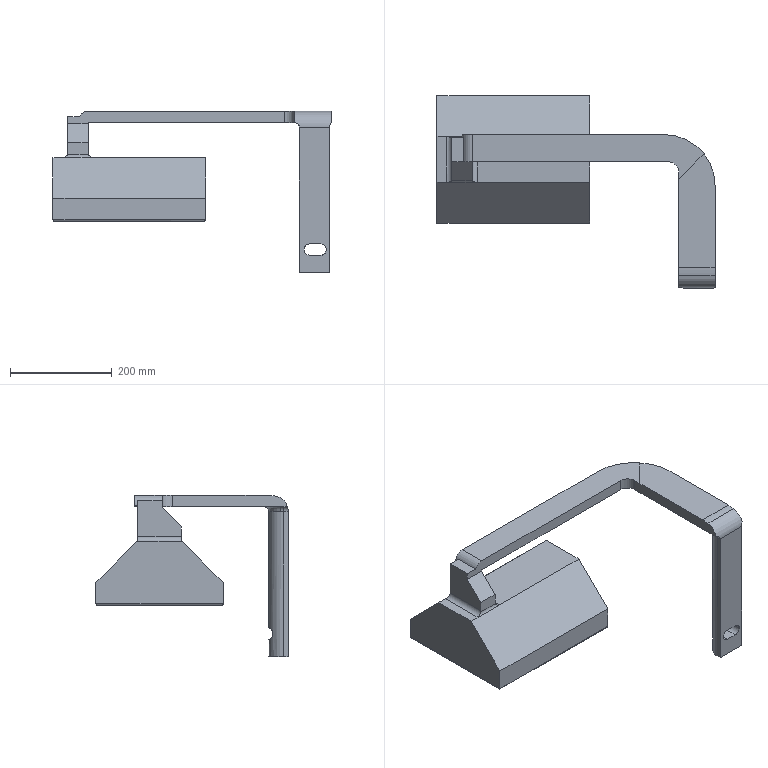Part | SolidWorks | features ICE 10, Fillet 8, Chamfer 2, Sweep 2, Extrusion 1 | 1 solid | 57 faces | box 546.764 x 377.712 x 317.016 mm | volume 9050376 mm3 | plane 35 | cylinder 19 | spline 2 | torus 1 | commonest cylinder face diameters 20 x6 6 x4 22 x3 40 x2 60 x2 160 x1